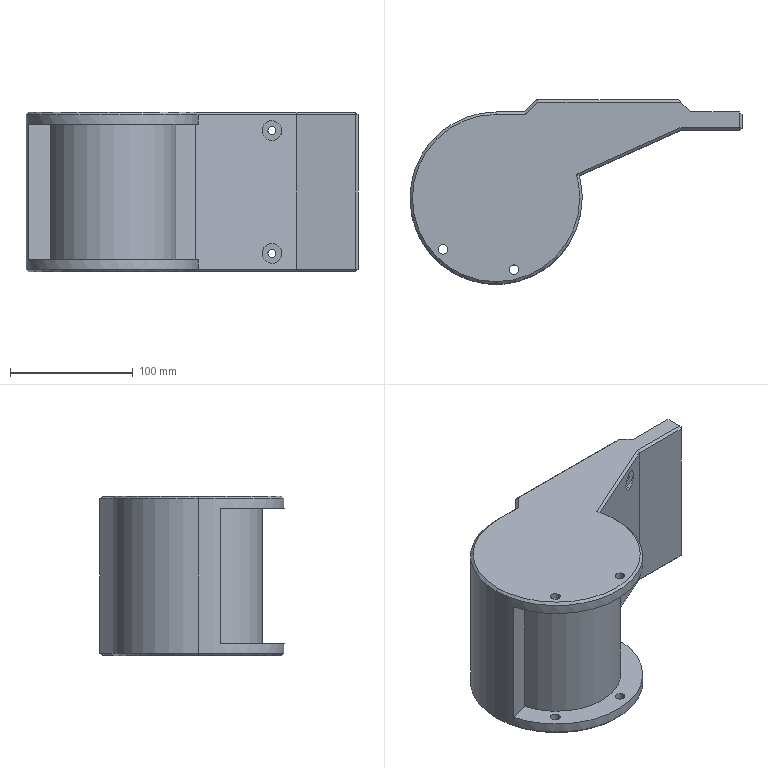Part | SolidWorks | features MirrorStock 1 | 1 solid | 62 faces | box 270 x 150 x 130 mm | volume 2349821 mm3 | plane 35 | cylinder 21 | cone 6 | commonest cylinder face diameters 8 x8 6.6 x4 16 x4 140 x4 104 x1